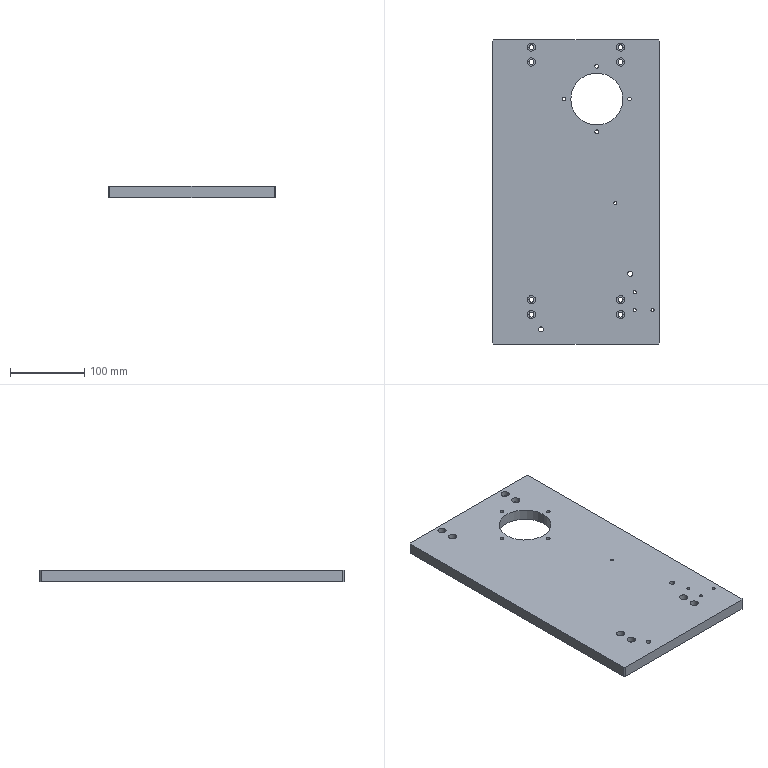Part | STEP file | 2005 Support shaft mounting plate | 1 solid | 75 faces | box 226 x 410 x 15 mm | volume 1321158 mm3 | cylinder 56 | plane 19 | commonest cylinder face diameters 6.6 x18 11 x18 4.2 x8 5 x8 6.8 x2 70 x2